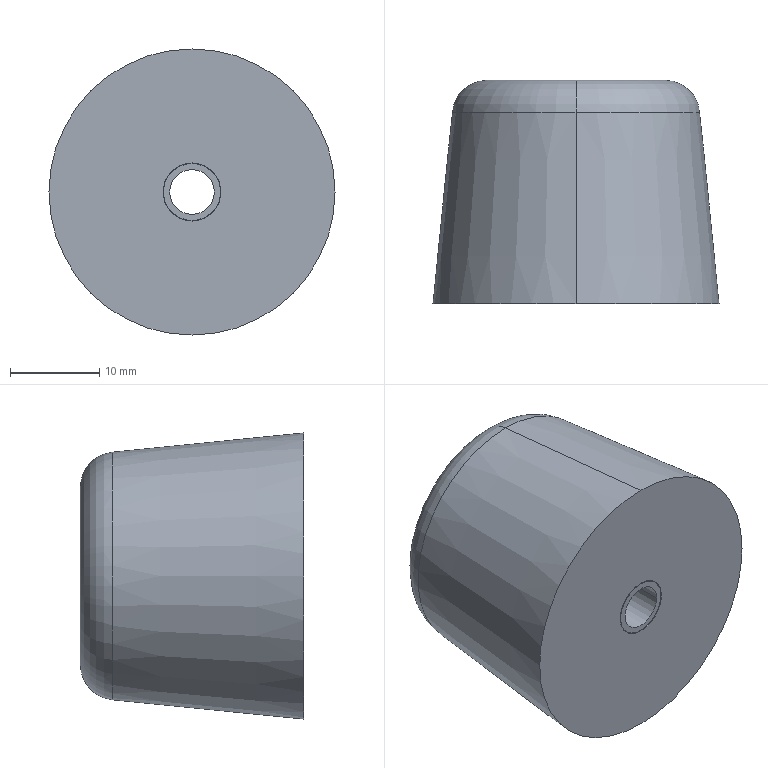Part | SolidWorks | features MBimport 1 | 1 solid | 17 faces | box 32 x 25 x 32 mm | volume 14674 mm3 | cylinder 8 | plane 5 | torus 2 | cone 2 | commonest cylinder face diameters 5 x2 6.4 x2 6.5 x2 14 x2
STEP:
#1=CARTESIAN_POINT('',(0.,25.,-9.88));
#2=VERTEX_POINT('',#1);
#3=CARTESIAN_POINT('',(0.,25.,9.88));
#4=VERTEX_POINT('',#3);
#5=CARTESIAN_POINT('',(0.,25.,0.));
#6=DIRECTION('',(0.,-1.,0.));
#7=DIRECTION('',(0.,0.,-1.));
#8=AXIS2_PLACEMENT_3D('',#5,#6,#7);
#9=CIRCLE('',#8,9.88);
#10=EDGE_CURVE('',#2,#4,#9,.T.);
#11=ORIENTED_EDGE('',*,*,#10,.T.);
#12=CARTESIAN_POINT('',(0.,21.398,13.86));
#13=VERTEX_POINT('',#12);
#14=CARTESIAN_POINT('',(0.,21.,9.88));
#15=DIRECTION('',(1.,0.,0.));
#16=DIRECTION('',(0.,0.,-1.));
#17=AXIS2_PLACEMENT_3D('',#14,#15,#16);
#18=CIRCLE('',#17,4.);
#19=EDGE_CURVE('',#4,#13,#18,.T.);
#20=ORIENTED_EDGE('',*,*,#19,.T.);
#21=CARTESIAN_POINT('',(0.,21.398,-13.86));
#22=VERTEX_POINT('',#21);
#23=CARTESIAN_POINT('',(0.,21.398,0.));
#24=DIRECTION('',(0.,-1.,0.));
#25=DIRECTION('',(0.,0.,-1.));
#26=AXIS2_PLACEMENT_3D('',#23,#24,#25);
#27=CIRCLE('',#26,13.86);
#28=EDGE_CURVE('',#22,#13,#27,.T.);
#29=ORIENTED_EDGE('',*,*,#28,.F.);
#30=CARTESIAN_POINT('',(0.,21.,-9.88));
#31=DIRECTION('',(-1.,0.,0.));
#32=DIRECTION('',(0.,0.,1.));
#33=AXIS2_PLACEMENT_3D('',#30,#31,#32);
#34=CIRCLE('',#33,4.);
#35=EDGE_CURVE('',#2,#22,#34,.T.);
#36=ORIENTED_EDGE('',*,*,#35,.F.);
#37=EDGE_LOOP('',(#11,#20,#29,#36));
#38=FACE_OUTER_BOUND('',#37,.T.);
#39=CARTESIAN_POINT('',(0.,21.,0.));
#40=DIRECTION('',(0.,-1.,0.));
#41=DIRECTION('',(0.,0.,-1.));
#42=AXIS2_PLACEMENT_3D('',#39,#40,#41);
#43=TOROIDAL_SURFACE('',#42,9.88,4.);
#44=ADVANCED_FACE('',(#38),#43,.T.);
#45=ORIENTED_EDGE('',*,*,#28,.T.);
#46=CARTESIAN_POINT('',(0.,0.,16.));
#47=VERTEX_POINT('',#46);
#48=CARTESIAN_POINT('',(0.,21.398,13.86));
#49=DIRECTION('',(0.,-0.995,0.0995));
#50=VECTOR('',#49,1000.);
#51=LINE('',#48,#50);
#52=EDGE_CURVE('',#13,#47,#51,.T.);
#53=ORIENTED_EDGE('',*,*,#52,.T.);
#54=CARTESIAN_POINT('',(0.,0.,-16.));
#55=VERTEX_POINT('',#54);
#56=CARTESIAN_POINT('',(0.,0.,0.));
#57=DIRECTION('',(0.,-1.,0.));
#58=DIRECTION('',(0.,0.,-1.));
#59=AXIS2_PLACEMENT_3D('',#56,#57,#58);
#60=CIRCLE('',#59,16.);
#61=EDGE_CURVE('',#55,#47,#60,.T.);
#62=ORIENTED_EDGE('',*,*,#61,.F.);
#63=CARTESIAN_POINT('',(0.,21.398,-13.86));
#64=DIRECTION('',(0.,-0.995,-0.0995));
#65=VECTOR('',#64,1000.);
#66=LINE('',#63,#65);
#67=EDGE_CURVE('',#22,#55,#66,.T.);
#68=ORIENTED_EDGE('',*,*,#67,.F.);
#69=EDGE_LOOP('',(#45,#53,#62,#68));
#70=FACE_OUTER_BOUND('',#69,.T.);
#71=CARTESIAN_POINT('',(0.,21.398,0.));
#72=DIRECTION('',(0.,-1.,0.));
#73=DIRECTION('',(0.,0.,-1.));
#74=AXIS2_PLACEMENT_3D('',#71,#72,#73);
#75=CONICAL_SURFACE('',#74,13.86,0.09967);
#76=ADVANCED_FACE('',(#70),#75,.T.);
#77=CARTESIAN_POINT('',(0.,0.05,3.25));
#78=VERTEX_POINT('',#77);
#79=CARTESIAN_POINT('',(0.,0.05,-3.25));
#80=VERTEX_POINT('',#79);
#81=CARTESIAN_POINT('',(0.,0.05,0.));
#82=DIRECTION('',(0.,-1.,0.));
#83=DIRECTION('',(0.,0.,-1.));
#84=AXIS2_PLACEMENT_3D('',#81,#82,#83);
#85=CIRCLE('',#84,3.25);
#86=EDGE_CURVE('',#78,#80,#85,.T.);
#87=ORIENTED_EDGE('',*,*,#86,.F.);
#88=CARTESIAN_POINT('',(0.,0.,3.25));
#89=VERTEX_POINT('',#88);
#90=CARTESIAN_POINT('',(0.,0.,3.25));
#91=DIRECTION('',(0.,-1.,0.));
#92=VECTOR('',#91,1000.);
#93=LINE('',#90,#92);
#94=EDGE_CURVE('',#78,#89,#93,.T.);
#95=ORIENTED_EDGE('',*,*,#94,.T.);
#96=CARTESIAN_POINT('',(0.,0.,-3.25));
#97=VERTEX_POINT('',#96);
#98=CARTESIAN_POINT('',(0.,0.,0.));
#99=DIRECTION('',(0.,-1.,0.));
#100=DIRECTION('',(0.,0.,-1.));
#101=AXIS2_PLACEMENT_3D('',#98,#99,#100);
#102=CIRCLE('',#101,3.25);
#103=EDGE_CURVE('',#89,#97,#102,.T.);
#104=ORIENTED_EDGE('',*,*,#103,.T.);
#105=CARTESIAN_POINT('',(0.,0.,-3.25));
#106=DIRECTION('',(0.,-1.,0.));
#107=VECTOR('',#106,1000.);
#108=LINE('',#105,#107);
#109=EDGE_CURVE('',#80,#97,#108,.T.);
#110=ORIENTED_EDGE('',*,*,#109,.F.);
#111=EDGE_LOOP('',(#87,#95,#104,#110));
#112=FACE_OUTER_BOUND('',#111,.T.);
#113=CARTESIAN_POINT('',(0.,0.,0.));
#114=DIRECTION('',(0.,-1.,0.));
#115=DIRECTION('',(0.,0.,-1.));
#116=AXIS2_PLACEMENT_3D('',#113,#114,#115);
#117=CYLINDRICAL_SURFACE('',#116,3.25);
#118=ADVANCED_FACE('',(#112),#117,.F.);
#119=CARTESIAN_POINT('',(0.,0.05,-3.2));
#120=VERTEX_POINT('',#119);
#121=CARTESIAN_POINT('',(0.,0.05,3.2));
#122=VERTEX_POINT('',#121);
#123=CARTESIAN_POINT('',(0.,0.05,0.));
#124=DIRECTION('',(0.,-1.,0.));
#125=DIRECTION('',(0.,0.,-1.));
#126=AXIS2_PLACEMENT_3D('',#123,#124,#125);
#127=CIRCLE('',#126,3.2);
#128=EDGE_CURVE('',#120,#122,#127,.T.);
#129=ORIENTED_EDGE('',*,*,#128,.T.);
#130=CARTESIAN_POINT('',(0.,0.,3.2));
#131=VERTEX_POINT('',#130);
#132=CARTESIAN_POINT('',(0.,0.,3.2));
#133=DIRECTION('',(0.,-1.,0.));
#134=VECTOR('',#133,1000.);
#135=LINE('',#132,#134);
#136=EDGE_CURVE('',#122,#131,#135,.T.);
#137=ORIENTED_EDGE('',*,*,#136,.T.);
#138=CARTESIAN_POINT('',(0.,0.,-3.2));
#139=VERTEX_POINT('',#138);
#140=CARTESIAN_POINT('',(0.,0.,0.));
#141=DIRECTION('',(0.,-1.,0.));
#142=DIRECTION('',(0.,0.,-1.));
#143=AXIS2_PLACEMENT_3D('',#140,#141,#142);
#144=CIRCLE('',#143,3.2);
#145=EDGE_CURVE('',#139,#131,#144,.T.);
#146=ORIENTED_EDGE('',*,*,#145,.F.);
#147=CARTESIAN_POINT('',(0.,0.,-3.2));
#148=DIRECTION('',(0.,-1.,0.));
#149=VECTOR('',#148,1000.);
#150=LINE('',#147,#149);
#151=EDGE_CURVE('',#120,#139,#150,.T.);
#152=ORIENTED_EDGE('',*,*,#151,.F.);
#153=EDGE_LOOP('',(#129,#137,#146,#152));
#154=FACE_OUTER_BOUND('',#153,.T.);
#155=CARTESIAN_POINT('',(0.,0.,0.));
#156=DIRECTION('',(0.,-1.,0.));
#157=DIRECTION('',(0.,0.,-1.));
#158=AXIS2_PLACEMENT_3D('',#155,#156,#157);
#159=CYLINDRICAL_SURFACE('',#158,3.2);
#160=ADVANCED_FACE('',(#154),#159,.T.);
#161=CARTESIAN_POINT('',(-7.,25.,0.));
#162=VERTEX_POINT('',#161);
#163=CARTESIAN_POINT('',(7.,25.,0.));
#164=VERTEX_POINT('',#163);
#165=CARTESIAN_POINT('',(0.,25.,0.));
#166=DIRECTION('',(0.,-1.,0.));
#167=DIRECTION('',(1.,0.,0.));
#168=AXIS2_PLACEMENT_3D('',#165,#166,#167);
#169=CIRCLE('',#168,7.);
#170=EDGE_CURVE('',#162,#164,#169,.T.);
#171=ORIENTED_EDGE('',*,*,#170,.F.);
#172=CARTESIAN_POINT('',(-7.,12.,0.));
#173=VERTEX_POINT('',#172);
#174=CARTESIAN_POINT('',(-7.,0.,0.));
#175=DIRECTION('',(0.,-1.,0.));
#176=VECTOR('',#175,1000.);
#177=LINE('',#174,#176);
#178=EDGE_CURVE('',#162,#173,#177,.T.);
#179=ORIENTED_EDGE('',*,*,#178,.T.);
#180=CARTESIAN_POINT('',(7.,12.,0.));
#181=VERTEX_POINT('',#180);
#182=CARTESIAN_POINT('',(0.,12.,0.));
#183=DIRECTION('',(0.,-1.,0.));
#184=DIRECTION('',(1.,0.,0.));
#185=AXIS2_PLACEMENT_3D('',#182,#183,#184);
#186=CIRCLE('',#185,7.);
#187=EDGE_CURVE('',#173,#181,#186,.T.);
#188=ORIENTED_EDGE('',*,*,#187,.T.);
#189=CARTESIAN_POINT('',(7.,0.,0.));
#190=DIRECTION('',(0.,-1.,0.));
#191=VECTOR('',#190,1000.);
#192=LINE('',#189,#191);
#193=EDGE_CURVE('',#164,#181,#192,.T.);
#194=ORIENTED_EDGE('',*,*,#193,.F.);
#195=EDGE_LOOP('',(#171,#179,#188,#194));
#196=FACE_OUTER_BOUND('',#195,.T.);
#197=CARTESIAN_POINT('',(0.,0.,0.));
#198=DIRECTION('',(0.,-1.,0.));
#199=DIRECTION('',(1.,0.,0.));
#200=AXIS2_PLACEMENT_3D('',#197,#198,#199);
#201=CYLINDRICAL_SURFACE('',#200,7.);
#202=ADVANCED_FACE('',(#196),#201,.F.);
#203=CARTESIAN_POINT('',(-2.5,12.,0.));
#204=VERTEX_POINT('',#203);
#205=CARTESIAN_POINT('',(2.5,12.,0.));
#206=VERTEX_POINT('',#205);
#207=CARTESIAN_POINT('',(0.,12.,0.));
#208=DIRECTION('',(0.,-1.,0.));
#209=DIRECTION('',(1.,0.,0.));
#210=AXIS2_PLACEMENT_3D('',#207,#208,#209);
#211=CIRCLE('',#210,2.5);
#212=EDGE_CURVE('',#204,#206,#211,.T.);
#213=ORIENTED_EDGE('',*,*,#212,.F.);
#214=CARTESIAN_POINT('',(-2.5,0.,0.));
#215=VERTEX_POINT('',#214);
#216=CARTESIAN_POINT('',(-2.5,0.,0.));
#217=DIRECTION('',(0.,-1.,0.));
#218=VECTOR('',#217,1000.);
#219=LINE('',#216,#218);
#220=EDGE_CURVE('',#204,#215,#219,.T.);
#221=ORIENTED_EDGE('',*,*,#220,.T.);
#222=CARTESIAN_POINT('',(2.5,0.,0.));
#223=VERTEX_POINT('',#222);
#224=CARTESIAN_POINT('',(0.,0.,0.));
#225=DIRECTION('',(0.,-1.,0.));
#226=DIRECTION('',(1.,0.,0.));
#227=AXIS2_PLACEMENT_3D('',#224,#225,#226);
#228=CIRCLE('',#227,2.5);
#229=EDGE_CURVE('',#215,#223,#228,.T.);
#230=ORIENTED_EDGE('',*,*,#229,.T.);
#231=CARTESIAN_POINT('',(2.5,0.,0.));
#232=DIRECTION('',(0.,-1.,0.));
#233=VECTOR('',#232,1000.);
#234=LINE('',#231,#233);
#235=EDGE_CURVE('',#206,#223,#234,.T.);
#236=ORIENTED_EDGE('',*,*,#235,.F.);
#237=EDGE_LOOP('',(#213,#221,#230,#236));
#238=FACE_OUTER_BOUND('',#237,.T.);
#239=CARTESIAN_POINT('',(0.,0.,0.));
#240=DIRECTION('',(0.,-1.,0.));
#241=DIRECTION('',(1.,0.,0.));
#242=AXIS2_PLACEMENT_3D('',#239,#240,#241);
#243=CYLINDRICAL_SURFACE('',#242,2.5);
#244=ADVANCED_FACE('',(#238),#243,.F.);
#245=ORIENTED_EDGE('',*,*,#220,.F.);
#246=CARTESIAN_POINT('',(0.,12.,0.));
#247=DIRECTION('',(0.,-1.,0.));
#248=DIRECTION('',(1.,0.,0.));
#249=AXIS2_PLACEMENT_3D('',#246,#247,#248);
#250=CIRCLE('',#249,2.5);
#251=EDGE_CURVE('',#206,#204,#250,.T.);
#252=ORIENTED_EDGE('',*,*,#251,.F.);
#253=ORIENTED_EDGE('',*,*,#235,.T.);
#254=CARTESIAN_POINT('',(0.,0.,0.));
#255=DIRECTION('',(0.,-1.,0.));
#256=DIRECTION('',(1.,0.,0.));
#257=AXIS2_PLACEMENT_3D('',#254,#255,#256);
#258=CIRCLE('',#257,2.5);
#259=EDGE_CURVE('',#223,#215,#258,.T.);
#260=ORIENTED_EDGE('',*,*,#259,.T.);
#261=EDGE_LOOP('',(#245,#252,#253,#260));
#262=FACE_OUTER_BOUND('',#261,.T.);
#263=CARTESIAN_POINT('',(0.,0.,0.));
#264=DIRECTION('',(0.,-1.,0.));
#265=DIRECTION('',(1.,0.,0.));
#266=AXIS2_PLACEMENT_3D('',#263,#264,#265);
#267=CYLINDRICAL_SURFACE('',#266,2.5);
#268=ADVANCED_FACE('',(#262),#267,.F.);
#269=CARTESIAN_POINT('',(0.,12.,0.));
#270=DIRECTION('',(0.,-1.,0.));
#271=DIRECTION('',(1.,0.,0.));
#272=AXIS2_PLACEMENT_3D('',#269,#270,#271);
#273=CIRCLE('',#272,7.);
#274=EDGE_CURVE('',#181,#173,#273,.T.);
#275=ORIENTED_EDGE('',*,*,#274,.F.);
#276=ORIENTED_EDGE('',*,*,#187,.F.);
#277=EDGE_LOOP('',(#275,#276));
#278=FACE_OUTER_BOUND('',#277,.T.);
#279=ORIENTED_EDGE('',*,*,#251,.T.);
#280=ORIENTED_EDGE('',*,*,#212,.T.);
#281=EDGE_LOOP('',(#279,#280));
#282=FACE_BOUND('',#281,.T.);
#283=CARTESIAN_POINT('',(7.,12.,0.));
#284=DIRECTION('',(0.,1.,0.));
#285=DIRECTION('',(1.,0.,0.));
#286=AXIS2_PLACEMENT_3D('',#283,#284,#285);
#287=PLANE('',#286);
#288=ADVANCED_FACE('',(#278,#282),#287,.T.);
#289=ORIENTED_EDGE('',*,*,#178,.F.);
#290=CARTESIAN_POINT('',(0.,25.,0.));
#291=DIRECTION('',(0.,-1.,0.));
#292=DIRECTION('',(1.,0.,0.));
#293=AXIS2_PLACEMENT_3D('',#290,#291,#292);
#294=CIRCLE('',#293,7.);
#295=EDGE_CURVE('',#164,#162,#294,.T.);
#296=ORIENTED_EDGE('',*,*,#295,.F.);
#297=ORIENTED_EDGE('',*,*,#193,.T.);
#298=ORIENTED_EDGE('',*,*,#274,.T.);
#299=EDGE_LOOP('',(#289,#296,#297,#298));
#300=FACE_OUTER_BOUND('',#299,.T.);
#301=CARTESIAN_POINT('',(0.,0.,0.));
#302=DIRECTION('',(0.,-1.,0.));
#303=DIRECTION('',(1.,0.,0.));
#304=AXIS2_PLACEMENT_3D('',#301,#302,#303);
#305=CYLINDRICAL_SURFACE('',#304,7.);
#306=ADVANCED_FACE('',(#300),#305,.F.);
#307=ORIENTED_EDGE('',*,*,#145,.T.);
#308=CARTESIAN_POINT('',(0.,0.,0.));
#309=DIRECTION('',(0.,-1.,0.));
#310=DIRECTION('',(0.,0.,-1.));
#311=AXIS2_PLACEMENT_3D('',#308,#309,#310);
#312=CIRCLE('',#311,3.2);
#313=EDGE_CURVE('',#131,#139,#312,.T.);
#314=ORIENTED_EDGE('',*,*,#313,.T.);
#315=EDGE_LOOP('',(#307,#314));
#316=FACE_OUTER_BOUND('',#315,.T.);
#317=ORIENTED_EDGE('',*,*,#259,.F.);
#318=ORIENTED_EDGE('',*,*,#229,.F.);
#319=EDGE_LOOP('',(#317,#318));
#320=FACE_BOUND('',#319,.T.);
#321=CARTESIAN_POINT('',(3.2,0.,0.));
#322=DIRECTION('',(0.,1.,0.));
#323=DIRECTION('',(1.,0.,0.));
#324=AXIS2_PLACEMENT_3D('',#321,#322,#323);
#325=PLANE('',#324);
#326=ADVANCED_FACE('',(#316,#320),#325,.F.);
#327=ORIENTED_EDGE('',*,*,#136,.F.);
#328=CARTESIAN_POINT('',(0.,0.05,0.));
#329=DIRECTION('',(0.,-1.,0.));
#330=DIRECTION('',(0.,0.,-1.));
#331=AXIS2_PLACEMENT_3D('',#328,#329,#330);
#332=CIRCLE('',#331,3.2);
#333=EDGE_CURVE('',#122,#120,#332,.T.);
#334=ORIENTED_EDGE('',*,*,#333,.T.);
#335=ORIENTED_EDGE('',*,*,#151,.T.);
#336=ORIENTED_EDGE('',*,*,#313,.F.);
#337=EDGE_LOOP('',(#327,#334,#335,#336));
#338=FACE_OUTER_BOUND('',#337,.T.);
#339=CARTESIAN_POINT('',(0.,0.,0.));
#340=DIRECTION('',(0.,-1.,0.));
#341=DIRECTION('',(0.,0.,-1.));
#342=AXIS2_PLACEMENT_3D('',#339,#340,#341);
#343=CYLINDRICAL_SURFACE('',#342,3.2);
#344=ADVANCED_FACE('',(#338),#343,.T.);
#345=CARTESIAN_POINT('',(0.,0.05,0.));
#346=DIRECTION('',(0.,-1.,0.));
#347=DIRECTION('',(0.,0.,-1.));
#348=AXIS2_PLACEMENT_3D('',#345,#346,#347);
#349=CIRCLE('',#348,3.25);
#350=EDGE_CURVE('',#80,#78,#349,.T.);
#351=ORIENTED_EDGE('',*,*,#350,.T.);
#352=ORIENTED_EDGE('',*,*,#86,.T.);
#353=EDGE_LOOP('',(#351,#352));
#354=FACE_OUTER_BOUND('',#353,.T.);
#355=ORIENTED_EDGE('',*,*,#128,.F.);
#356=ORIENTED_EDGE('',*,*,#333,.F.);
#357=EDGE_LOOP('',(#355,#356));
#358=FACE_BOUND('',#357,.T.);
#359=CARTESIAN_POINT('',(3.25,0.05,0.));
#360=DIRECTION('',(0.,1.,0.));
#361=DIRECTION('',(1.,0.,0.));
#362=AXIS2_PLACEMENT_3D('',#359,#360,#361);
#363=PLANE('',#362);
#364=ADVANCED_FACE('',(#354,#358),#363,.F.);
#365=ORIENTED_EDGE('',*,*,#94,.F.);
#366=ORIENTED_EDGE('',*,*,#350,.F.);
#367=ORIENTED_EDGE('',*,*,#109,.T.);
#368=CARTESIAN_POINT('',(0.,0.,0.));
#369=DIRECTION('',(0.,-1.,0.));
#370=DIRECTION('',(0.,0.,-1.));
#371=AXIS2_PLACEMENT_3D('',#368,#369,#370);
#372=CIRCLE('',#371,3.25);
#373=EDGE_CURVE('',#97,#89,#372,.T.);
#374=ORIENTED_EDGE('',*,*,#373,.T.);
#375=EDGE_LOOP('',(#365,#366,#367,#374));
#376=FACE_OUTER_BOUND('',#375,.T.);
#377=CARTESIAN_POINT('',(0.,0.,0.));
#378=DIRECTION('',(0.,-1.,0.));
#379=DIRECTION('',(0.,0.,-1.));
#380=AXIS2_PLACEMENT_3D('',#377,#378,#379);
#381=CYLINDRICAL_SURFACE('',#380,3.25);
#382=ADVANCED_FACE('',(#376),#381,.F.);
#383=ORIENTED_EDGE('',*,*,#61,.T.);
#384=CARTESIAN_POINT('',(0.,0.,0.));
#385=DIRECTION('',(0.,-1.,0.));
#386=DIRECTION('',(0.,0.,-1.));
#387=AXIS2_PLACEMENT_3D('',#384,#385,#386);
#388=CIRCLE('',#387,16.);
#389=EDGE_CURVE('',#47,#55,#388,.T.);
#390=ORIENTED_EDGE('',*,*,#389,.T.);
#391=EDGE_LOOP('',(#383,#390));
#392=FACE_OUTER_BOUND('',#391,.T.);
#393=ORIENTED_EDGE('',*,*,#373,.F.);
#394=ORIENTED_EDGE('',*,*,#103,.F.);
#395=EDGE_LOOP('',(#393,#394));
#396=FACE_BOUND('',#395,.T.);
#397=CARTESIAN_POINT('',(16.,0.,0.));
#398=DIRECTION('',(0.,1.,0.));
#399=DIRECTION('',(1.,0.,0.));
#400=AXIS2_PLACEMENT_3D('',#397,#398,#399);
#401=PLANE('',#400);
#402=ADVANCED_FACE('',(#392,#396),#401,.F.);
#403=ORIENTED_EDGE('',*,*,#52,.F.);
#404=CARTESIAN_POINT('',(0.,21.398,0.));
#405=DIRECTION('',(0.,-1.,0.));
#406=DIRECTION('',(0.,0.,-1.));
#407=AXIS2_PLACEMENT_3D('',#404,#405,#406);
#408=CIRCLE('',#407,13.86);
#409=EDGE_CURVE('',#13,#22,#408,.T.);
#410=ORIENTED_EDGE('',*,*,#409,.T.);
#411=ORIENTED_EDGE('',*,*,#67,.T.);
#412=ORIENTED_EDGE('',*,*,#389,.F.);
#413=EDGE_LOOP('',(#403,#410,#411,#412));
#414=FACE_OUTER_BOUND('',#413,.T.);
#415=CARTESIAN_POINT('',(0.,21.398,0.));
#416=DIRECTION('',(0.,-1.,0.));
#417=DIRECTION('',(0.,0.,-1.));
#418=AXIS2_PLACEMENT_3D('',#415,#416,#417);
#419=CONICAL_SURFACE('',#418,13.86,0.09967);
#420=ADVANCED_FACE('',(#414),#419,.T.);
#421=ORIENTED_EDGE('',*,*,#19,.F.);
#422=CARTESIAN_POINT('',(0.,25.,0.));
#423=DIRECTION('',(0.,-1.,0.));
#424=DIRECTION('',(0.,0.,-1.));
#425=AXIS2_PLACEMENT_3D('',#422,#423,#424);
#426=CIRCLE('',#425,9.88);
#427=EDGE_CURVE('',#4,#2,#426,.T.);
#428=ORIENTED_EDGE('',*,*,#427,.T.);
#429=ORIENTED_EDGE('',*,*,#35,.T.);
#430=ORIENTED_EDGE('',*,*,#409,.F.);
#431=EDGE_LOOP('',(#421,#428,#429,#430));
#432=FACE_OUTER_BOUND('',#431,.T.);
#433=CARTESIAN_POINT('',(0.,21.,0.));
#434=DIRECTION('',(0.,-1.,0.));
#435=DIRECTION('',(0.,0.,-1.));
#436=AXIS2_PLACEMENT_3D('',#433,#434,#435);
#437=TOROIDAL_SURFACE('',#436,9.88,4.);
#438=ADVANCED_FACE('',(#432),#437,.T.);
#439=ORIENTED_EDGE('',*,*,#295,.T.);
#440=ORIENTED_EDGE('',*,*,#170,.T.);
#441=EDGE_LOOP('',(#439,#440));
#442=FACE_BOUND('',#441,.T.);
#443=ORIENTED_EDGE('',*,*,#10,.F.);
#444=ORIENTED_EDGE('',*,*,#427,.F.);
#445=EDGE_LOOP('',(#443,#444));
#446=FACE_OUTER_BOUND('',#445,.T.);
#447=CARTESIAN_POINT('',(0.,25.,0.));
#448=DIRECTION('',(0.,-1.,0.));
#449=DIRECTION('',(0.,0.,-1.));
#450=AXIS2_PLACEMENT_3D('',#447,#448,#449);
#451=PLANE('',#450);
#452=ADVANCED_FACE('',(#442,#446),#451,.F.);
#453=CLOSED_SHELL('',(#44,#76,#118,#160,#202,#244,#268,#288,#306,#326,#344,#364,#382,#402,#420,#438,#452));
#454=MANIFOLD_SOLID_BREP('',#453);
#455=CARTESIAN_POINT('',(0.,0.,0.));
#456=DIRECTION('',(0.,0.,1.));
#457=DIRECTION('',(1.,0.,0.));
#458=AXIS2_PLACEMENT_3D('',#455,#456,#457);
#459=(LENGTH_UNIT()NAMED_UNIT(*)SI_UNIT(.MILLI.,.METRE.));
#460=UNCERTAINTY_MEASURE_WITH_UNIT(LENGTH_MEASURE(0.00001),#459,'','');
#461=(NAMED_UNIT(*)PLANE_ANGLE_UNIT()SI_UNIT($,.RADIAN.));
#462=(NAMED_UNIT(*)SI_UNIT($,.STERADIAN.)SOLID_ANGLE_UNIT());
#463=(GEOMETRIC_REPRESENTATION_CONTEXT(3)GLOBAL_UNCERTAINTY_ASSIGNED_CONTEXT((#460))GLOBAL_UNIT_ASSIGNED_CONTEXT((#459,#461,#462))REPRESENTATION_CONTEXT('',''));
#464=ADVANCED_BREP_SHAPE_REPRESENTATION('',(#454,#458),#463);